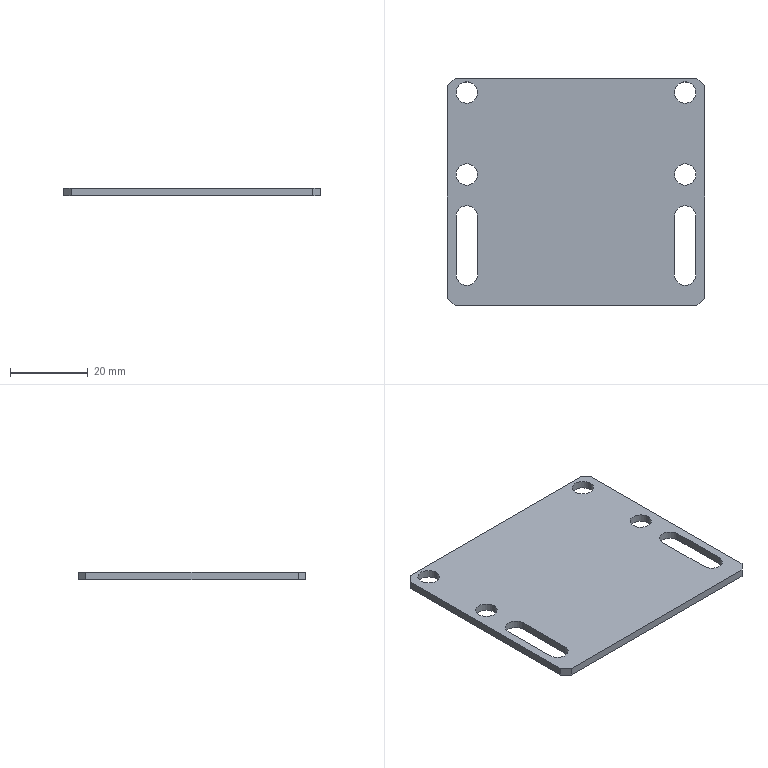Part | STEP file | PN_0001-01-12 Sensor board | 1 solid | 26 faces | box 66 x 58.5 x 2 mm | volume 7091 mm3 | plane 14 | cylinder 12 | commonest cylinder face diameters 5.5 x12
STEP:
#1=CARTESIAN_POINT('',(30.75,4.5,0.));
#2=VERTEX_POINT('',#1);
#3=CARTESIAN_POINT('',(25.25,4.5,0.));
#4=VERTEX_POINT('',#3);
#5=CARTESIAN_POINT('',(28.,4.5,0.));
#6=DIRECTION('',(0.,0.,-1.));
#7=DIRECTION('',(1.,0.,0.));
#8=AXIS2_PLACEMENT_3D('',#5,#6,#7);
#9=CIRCLE('',#8,2.75);
#10=EDGE_CURVE('',#2,#4,#9,.T.);
#11=ORIENTED_EDGE('',*,*,#10,.T.);
#12=CARTESIAN_POINT('',(25.25,4.5,2.));
#13=VERTEX_POINT('',#12);
#14=CARTESIAN_POINT('',(25.25,4.5,-0.001));
#15=DIRECTION('',(0.,0.,1.));
#16=VECTOR('',#15,1000.);
#17=LINE('',#14,#16);
#18=EDGE_CURVE('',#4,#13,#17,.T.);
#19=ORIENTED_EDGE('',*,*,#18,.T.);
#20=CARTESIAN_POINT('',(30.75,4.5,2.));
#21=VERTEX_POINT('',#20);
#22=CARTESIAN_POINT('',(28.,4.5,2.));
#23=DIRECTION('',(0.,0.,1.));
#24=DIRECTION('',(1.,0.,0.));
#25=AXIS2_PLACEMENT_3D('',#22,#23,#24);
#26=CIRCLE('',#25,2.75);
#27=EDGE_CURVE('',#13,#21,#26,.T.);
#28=ORIENTED_EDGE('',*,*,#27,.T.);
#29=CARTESIAN_POINT('',(30.75,4.5,-0.001));
#30=DIRECTION('',(0.,0.,1.));
#31=VECTOR('',#30,1000.);
#32=LINE('',#29,#31);
#33=EDGE_CURVE('',#2,#21,#32,.T.);
#34=ORIENTED_EDGE('',*,*,#33,.F.);
#35=EDGE_LOOP('',(#11,#19,#28,#34));
#36=FACE_OUTER_BOUND('',#35,.T.);
#37=CARTESIAN_POINT('',(28.,4.5,-0.001));
#38=DIRECTION('',(0.,0.,1.));
#39=DIRECTION('',(1.,0.,0.));
#40=AXIS2_PLACEMENT_3D('',#37,#38,#39);
#41=CYLINDRICAL_SURFACE('',#40,2.75);
#42=ADVANCED_FACE('',(#36),#41,.F.);
#43=CARTESIAN_POINT('',(-25.25,4.5,0.));
#44=VERTEX_POINT('',#43);
#45=CARTESIAN_POINT('',(-30.75,4.5,0.));
#46=VERTEX_POINT('',#45);
#47=CARTESIAN_POINT('',(-28.,4.5,0.));
#48=DIRECTION('',(0.,0.,-1.));
#49=DIRECTION('',(1.,0.,0.));
#50=AXIS2_PLACEMENT_3D('',#47,#48,#49);
#51=CIRCLE('',#50,2.75);
#52=EDGE_CURVE('',#44,#46,#51,.T.);
#53=ORIENTED_EDGE('',*,*,#52,.T.);
#54=CARTESIAN_POINT('',(-30.75,4.5,2.));
#55=VERTEX_POINT('',#54);
#56=CARTESIAN_POINT('',(-30.75,4.5,-0.001));
#57=DIRECTION('',(0.,0.,1.));
#58=VECTOR('',#57,1000.);
#59=LINE('',#56,#58);
#60=EDGE_CURVE('',#46,#55,#59,.T.);
#61=ORIENTED_EDGE('',*,*,#60,.T.);
#62=CARTESIAN_POINT('',(-25.25,4.5,2.));
#63=VERTEX_POINT('',#62);
#64=CARTESIAN_POINT('',(-28.,4.5,2.));
#65=DIRECTION('',(0.,0.,1.));
#66=DIRECTION('',(1.,0.,0.));
#67=AXIS2_PLACEMENT_3D('',#64,#65,#66);
#68=CIRCLE('',#67,2.75);
#69=EDGE_CURVE('',#55,#63,#68,.T.);
#70=ORIENTED_EDGE('',*,*,#69,.T.);
#71=CARTESIAN_POINT('',(-25.25,4.5,-0.001));
#72=DIRECTION('',(0.,0.,1.));
#73=VECTOR('',#72,1000.);
#74=LINE('',#71,#73);
#75=EDGE_CURVE('',#44,#63,#74,.T.);
#76=ORIENTED_EDGE('',*,*,#75,.F.);
#77=EDGE_LOOP('',(#53,#61,#70,#76));
#78=FACE_OUTER_BOUND('',#77,.T.);
#79=CARTESIAN_POINT('',(-28.,4.5,-0.001));
#80=DIRECTION('',(0.,0.,1.));
#81=DIRECTION('',(1.,0.,0.));
#82=AXIS2_PLACEMENT_3D('',#79,#80,#81);
#83=CYLINDRICAL_SURFACE('',#82,2.75);
#84=ADVANCED_FACE('',(#78),#83,.F.);
#85=CARTESIAN_POINT('',(30.75,25.5,0.));
#86=VERTEX_POINT('',#85);
#87=CARTESIAN_POINT('',(25.25,25.5,0.));
#88=VERTEX_POINT('',#87);
#89=CARTESIAN_POINT('',(28.,25.5,0.));
#90=DIRECTION('',(0.,0.,-1.));
#91=DIRECTION('',(1.,0.,0.));
#92=AXIS2_PLACEMENT_3D('',#89,#90,#91);
#93=CIRCLE('',#92,2.75);
#94=EDGE_CURVE('',#86,#88,#93,.T.);
#95=ORIENTED_EDGE('',*,*,#94,.T.);
#96=CARTESIAN_POINT('',(25.25,25.5,2.));
#97=VERTEX_POINT('',#96);
#98=CARTESIAN_POINT('',(25.25,25.5,-0.001));
#99=DIRECTION('',(0.,0.,1.));
#100=VECTOR('',#99,1000.);
#101=LINE('',#98,#100);
#102=EDGE_CURVE('',#88,#97,#101,.T.);
#103=ORIENTED_EDGE('',*,*,#102,.T.);
#104=CARTESIAN_POINT('',(30.75,25.5,2.));
#105=VERTEX_POINT('',#104);
#106=CARTESIAN_POINT('',(28.,25.5,2.));
#107=DIRECTION('',(0.,0.,1.));
#108=DIRECTION('',(1.,0.,0.));
#109=AXIS2_PLACEMENT_3D('',#106,#107,#108);
#110=CIRCLE('',#109,2.75);
#111=EDGE_CURVE('',#97,#105,#110,.T.);
#112=ORIENTED_EDGE('',*,*,#111,.T.);
#113=CARTESIAN_POINT('',(30.75,25.5,-0.001));
#114=DIRECTION('',(0.,0.,1.));
#115=VECTOR('',#114,1000.);
#116=LINE('',#113,#115);
#117=EDGE_CURVE('',#86,#105,#116,.T.);
#118=ORIENTED_EDGE('',*,*,#117,.F.);
#119=EDGE_LOOP('',(#95,#103,#112,#118));
#120=FACE_OUTER_BOUND('',#119,.T.);
#121=CARTESIAN_POINT('',(28.,25.5,-0.001));
#122=DIRECTION('',(0.,0.,1.));
#123=DIRECTION('',(1.,0.,0.));
#124=AXIS2_PLACEMENT_3D('',#121,#122,#123);
#125=CYLINDRICAL_SURFACE('',#124,2.75);
#126=ADVANCED_FACE('',(#120),#125,.F.);
#127=CARTESIAN_POINT('',(-25.25,25.5,0.));
#128=VERTEX_POINT('',#127);
#129=CARTESIAN_POINT('',(-30.75,25.5,0.));
#130=VERTEX_POINT('',#129);
#131=CARTESIAN_POINT('',(-28.,25.5,0.));
#132=DIRECTION('',(0.,0.,-1.));
#133=DIRECTION('',(1.,0.,0.));
#134=AXIS2_PLACEMENT_3D('',#131,#132,#133);
#135=CIRCLE('',#134,2.75);
#136=EDGE_CURVE('',#128,#130,#135,.T.);
#137=ORIENTED_EDGE('',*,*,#136,.T.);
#138=CARTESIAN_POINT('',(-30.75,25.5,2.));
#139=VERTEX_POINT('',#138);
#140=CARTESIAN_POINT('',(-30.75,25.5,-0.001));
#141=DIRECTION('',(0.,0.,1.));
#142=VECTOR('',#141,1000.);
#143=LINE('',#140,#142);
#144=EDGE_CURVE('',#130,#139,#143,.T.);
#145=ORIENTED_EDGE('',*,*,#144,.T.);
#146=CARTESIAN_POINT('',(-25.25,25.5,2.));
#147=VERTEX_POINT('',#146);
#148=CARTESIAN_POINT('',(-28.,25.5,2.));
#149=DIRECTION('',(0.,0.,1.));
#150=DIRECTION('',(1.,0.,0.));
#151=AXIS2_PLACEMENT_3D('',#148,#149,#150);
#152=CIRCLE('',#151,2.75);
#153=EDGE_CURVE('',#139,#147,#152,.T.);
#154=ORIENTED_EDGE('',*,*,#153,.T.);
#155=CARTESIAN_POINT('',(-25.25,25.5,-0.001));
#156=DIRECTION('',(0.,0.,1.));
#157=VECTOR('',#156,1000.);
#158=LINE('',#155,#157);
#159=EDGE_CURVE('',#128,#147,#158,.T.);
#160=ORIENTED_EDGE('',*,*,#159,.F.);
#161=EDGE_LOOP('',(#137,#145,#154,#160));
#162=FACE_OUTER_BOUND('',#161,.T.);
#163=CARTESIAN_POINT('',(-28.,25.5,-0.001));
#164=DIRECTION('',(0.,0.,1.));
#165=DIRECTION('',(1.,0.,0.));
#166=AXIS2_PLACEMENT_3D('',#163,#164,#165);
#167=CYLINDRICAL_SURFACE('',#166,2.75);
#168=ADVANCED_FACE('',(#162),#167,.F.);
#169=CARTESIAN_POINT('',(25.25,-21.25,0.));
#170=VERTEX_POINT('',#169);
#171=CARTESIAN_POINT('',(25.25,-21.25,2.));
#172=VERTEX_POINT('',#171);
#173=CARTESIAN_POINT('',(25.25,-21.25,-0.001));
#174=DIRECTION('',(0.,0.,1.));
#175=VECTOR('',#174,1000.);
#176=LINE('',#173,#175);
#177=EDGE_CURVE('',#170,#172,#176,.T.);
#178=ORIENTED_EDGE('',*,*,#177,.T.);
#179=CARTESIAN_POINT('',(30.75,-21.25,2.));
#180=VERTEX_POINT('',#179);
#181=CARTESIAN_POINT('',(28.,-21.25,2.));
#182=DIRECTION('',(0.,0.,1.));
#183=DIRECTION('',(1.,0.,0.));
#184=AXIS2_PLACEMENT_3D('',#181,#182,#183);
#185=CIRCLE('',#184,2.75);
#186=EDGE_CURVE('',#172,#180,#185,.T.);
#187=ORIENTED_EDGE('',*,*,#186,.T.);
#188=CARTESIAN_POINT('',(30.75,-21.25,0.));
#189=VERTEX_POINT('',#188);
#190=CARTESIAN_POINT('',(30.75,-21.25,-0.001));
#191=DIRECTION('',(0.,0.,1.));
#192=VECTOR('',#191,1000.);
#193=LINE('',#190,#192);
#194=EDGE_CURVE('',#189,#180,#193,.T.);
#195=ORIENTED_EDGE('',*,*,#194,.F.);
#196=CARTESIAN_POINT('',(28.,-21.25,0.));
#197=DIRECTION('',(0.,0.,-1.));
#198=DIRECTION('',(1.,0.,0.));
#199=AXIS2_PLACEMENT_3D('',#196,#197,#198);
#200=CIRCLE('',#199,2.75);
#201=EDGE_CURVE('',#189,#170,#200,.T.);
#202=ORIENTED_EDGE('',*,*,#201,.T.);
#203=EDGE_LOOP('',(#178,#187,#195,#202));
#204=FACE_OUTER_BOUND('',#203,.T.);
#205=CARTESIAN_POINT('',(28.,-21.25,-0.001));
#206=DIRECTION('',(0.,0.,1.));
#207=DIRECTION('',(1.,0.,0.));
#208=AXIS2_PLACEMENT_3D('',#205,#206,#207);
#209=CYLINDRICAL_SURFACE('',#208,2.75);
#210=ADVANCED_FACE('',(#204),#209,.F.);
#211=CARTESIAN_POINT('',(-30.75,-21.25,0.));
#212=VERTEX_POINT('',#211);
#213=CARTESIAN_POINT('',(-30.75,-21.25,2.));
#214=VERTEX_POINT('',#213);
#215=CARTESIAN_POINT('',(-30.75,-21.25,-0.001));
#216=DIRECTION('',(0.,0.,1.));
#217=VECTOR('',#216,1000.);
#218=LINE('',#215,#217);
#219=EDGE_CURVE('',#212,#214,#218,.T.);
#220=ORIENTED_EDGE('',*,*,#219,.T.);
#221=CARTESIAN_POINT('',(-25.25,-21.25,2.));
#222=VERTEX_POINT('',#221);
#223=CARTESIAN_POINT('',(-28.,-21.25,2.));
#224=DIRECTION('',(0.,0.,1.));
#225=DIRECTION('',(1.,0.,0.));
#226=AXIS2_PLACEMENT_3D('',#223,#224,#225);
#227=CIRCLE('',#226,2.75);
#228=EDGE_CURVE('',#214,#222,#227,.T.);
#229=ORIENTED_EDGE('',*,*,#228,.T.);
#230=CARTESIAN_POINT('',(-25.25,-21.25,0.));
#231=VERTEX_POINT('',#230);
#232=CARTESIAN_POINT('',(-25.25,-21.25,-0.001));
#233=DIRECTION('',(0.,0.,1.));
#234=VECTOR('',#233,1000.);
#235=LINE('',#232,#234);
#236=EDGE_CURVE('',#231,#222,#235,.T.);
#237=ORIENTED_EDGE('',*,*,#236,.F.);
#238=CARTESIAN_POINT('',(-28.,-21.25,0.));
#239=DIRECTION('',(0.,0.,-1.));
#240=DIRECTION('',(1.,0.,0.));
#241=AXIS2_PLACEMENT_3D('',#238,#239,#240);
#242=CIRCLE('',#241,2.75);
#243=EDGE_CURVE('',#231,#212,#242,.T.);
#244=ORIENTED_EDGE('',*,*,#243,.T.);
#245=EDGE_LOOP('',(#220,#229,#237,#244));
#246=FACE_OUTER_BOUND('',#245,.T.);
#247=CARTESIAN_POINT('',(-28.,-21.25,-0.001));
#248=DIRECTION('',(0.,0.,1.));
#249=DIRECTION('',(1.,0.,0.));
#250=AXIS2_PLACEMENT_3D('',#247,#248,#249);
#251=CYLINDRICAL_SURFACE('',#250,2.75);
#252=ADVANCED_FACE('',(#246),#251,.F.);
#253=CARTESIAN_POINT('',(-33.,27.25,0.));
#254=VERTEX_POINT('',#253);
#255=CARTESIAN_POINT('',(-33.,-27.25,0.));
#256=VERTEX_POINT('',#255);
#257=CARTESIAN_POINT('',(-33.,-29.25,0.));
#258=DIRECTION('',(0.,-1.,0.));
#259=VECTOR('',#258,1000.);
#260=LINE('',#257,#259);
#261=EDGE_CURVE('',#254,#256,#260,.T.);
#262=ORIENTED_EDGE('',*,*,#261,.T.);
#263=CARTESIAN_POINT('',(-33.,-27.25,2.));
#264=VERTEX_POINT('',#263);
#265=CARTESIAN_POINT('',(-33.,-27.25,2.));
#266=DIRECTION('',(0.,0.,1.));
#267=VECTOR('',#266,1000.);
#268=LINE('',#265,#267);
#269=EDGE_CURVE('',#256,#264,#268,.T.);
#270=ORIENTED_EDGE('',*,*,#269,.T.);
#271=CARTESIAN_POINT('',(-33.,27.25,2.));
#272=VERTEX_POINT('',#271);
#273=CARTESIAN_POINT('',(-33.,-29.25,2.));
#274=DIRECTION('',(0.,-1.,0.));
#275=VECTOR('',#274,1000.);
#276=LINE('',#273,#275);
#277=EDGE_CURVE('',#272,#264,#276,.T.);
#278=ORIENTED_EDGE('',*,*,#277,.F.);
#279=CARTESIAN_POINT('',(-33.,27.25,2.));
#280=DIRECTION('',(0.,0.,-1.));
#281=VECTOR('',#280,1000.);
#282=LINE('',#279,#281);
#283=EDGE_CURVE('',#272,#254,#282,.T.);
#284=ORIENTED_EDGE('',*,*,#283,.T.);
#285=EDGE_LOOP('',(#262,#270,#278,#284));
#286=FACE_OUTER_BOUND('',#285,.T.);
#287=CARTESIAN_POINT('',(-33.,-29.25,2.));
#288=DIRECTION('',(1.,0.,0.));
#289=DIRECTION('',(0.,0.,-1.));
#290=AXIS2_PLACEMENT_3D('',#287,#288,#289);
#291=PLANE('',#290);
#292=ADVANCED_FACE('',(#286),#291,.F.);
#293=CARTESIAN_POINT('',(-31.,-29.25,2.));
#294=VERTEX_POINT('',#293);
#295=CARTESIAN_POINT('',(31.,-29.25,2.));
#296=VERTEX_POINT('',#295);
#297=CARTESIAN_POINT('',(33.,-29.25,2.));
#298=DIRECTION('',(1.,0.,0.));
#299=VECTOR('',#298,1000.);
#300=LINE('',#297,#299);
#301=EDGE_CURVE('',#294,#296,#300,.T.);
#302=ORIENTED_EDGE('',*,*,#301,.F.);
#303=CARTESIAN_POINT('',(-31.,-29.25,0.));
#304=VERTEX_POINT('',#303);
#305=CARTESIAN_POINT('',(-31.,-29.25,2.));
#306=DIRECTION('',(0.,0.,-1.));
#307=VECTOR('',#306,1000.);
#308=LINE('',#305,#307);
#309=EDGE_CURVE('',#294,#304,#308,.T.);
#310=ORIENTED_EDGE('',*,*,#309,.T.);
#311=CARTESIAN_POINT('',(31.,-29.25,0.));
#312=VERTEX_POINT('',#311);
#313=CARTESIAN_POINT('',(33.,-29.25,0.));
#314=DIRECTION('',(1.,0.,0.));
#315=VECTOR('',#314,1000.);
#316=LINE('',#313,#315);
#317=EDGE_CURVE('',#304,#312,#316,.T.);
#318=ORIENTED_EDGE('',*,*,#317,.T.);
#319=CARTESIAN_POINT('',(31.,-29.25,2.));
#320=DIRECTION('',(0.,0.,1.));
#321=VECTOR('',#320,1000.);
#322=LINE('',#319,#321);
#323=EDGE_CURVE('',#312,#296,#322,.T.);
#324=ORIENTED_EDGE('',*,*,#323,.T.);
#325=EDGE_LOOP('',(#302,#310,#318,#324));
#326=FACE_OUTER_BOUND('',#325,.T.);
#327=CARTESIAN_POINT('',(33.,-29.25,2.));
#328=DIRECTION('',(0.,1.,0.));
#329=DIRECTION('',(-1.,0.,0.));
#330=AXIS2_PLACEMENT_3D('',#327,#328,#329);
#331=PLANE('',#330);
#332=ADVANCED_FACE('',(#326),#331,.F.);
#333=CARTESIAN_POINT('',(33.,-27.25,2.));
#334=VERTEX_POINT('',#333);
#335=CARTESIAN_POINT('',(33.,27.25,2.));
#336=VERTEX_POINT('',#335);
#337=CARTESIAN_POINT('',(33.,-29.25,2.));
#338=DIRECTION('',(0.,1.,0.));
#339=VECTOR('',#338,1000.);
#340=LINE('',#337,#339);
#341=EDGE_CURVE('',#334,#336,#340,.T.);
#342=ORIENTED_EDGE('',*,*,#341,.F.);
#343=CARTESIAN_POINT('',(33.,-27.25,0.));
#344=VERTEX_POINT('',#343);
#345=CARTESIAN_POINT('',(33.,-27.25,2.));
#346=DIRECTION('',(0.,0.,-1.));
#347=VECTOR('',#346,1000.);
#348=LINE('',#345,#347);
#349=EDGE_CURVE('',#334,#344,#348,.T.);
#350=ORIENTED_EDGE('',*,*,#349,.T.);
#351=CARTESIAN_POINT('',(33.,27.25,0.));
#352=VERTEX_POINT('',#351);
#353=CARTESIAN_POINT('',(33.,-29.25,0.));
#354=DIRECTION('',(0.,1.,0.));
#355=VECTOR('',#354,1000.);
#356=LINE('',#353,#355);
#357=EDGE_CURVE('',#344,#352,#356,.T.);
#358=ORIENTED_EDGE('',*,*,#357,.T.);
#359=CARTESIAN_POINT('',(33.,27.25,2.));
#360=DIRECTION('',(0.,0.,1.));
#361=VECTOR('',#360,1000.);
#362=LINE('',#359,#361);
#363=EDGE_CURVE('',#352,#336,#362,.T.);
#364=ORIENTED_EDGE('',*,*,#363,.T.);
#365=EDGE_LOOP('',(#342,#350,#358,#364));
#366=FACE_OUTER_BOUND('',#365,.T.);
#367=CARTESIAN_POINT('',(33.,-29.25,2.));
#368=DIRECTION('',(-1.,0.,0.));
#369=DIRECTION('',(0.,0.,1.));
#370=AXIS2_PLACEMENT_3D('',#367,#368,#369);
#371=PLANE('',#370);
#372=ADVANCED_FACE('',(#366),#371,.F.);
#373=CARTESIAN_POINT('',(31.,29.25,0.));
#374=VERTEX_POINT('',#373);
#375=CARTESIAN_POINT('',(-31.,29.25,0.));
#376=VERTEX_POINT('',#375);
#377=CARTESIAN_POINT('',(33.,29.25,0.));
#378=DIRECTION('',(-1.,0.,0.));
#379=VECTOR('',#378,1000.);
#380=LINE('',#377,#379);
#381=EDGE_CURVE('',#374,#376,#380,.T.);
#382=ORIENTED_EDGE('',*,*,#381,.T.);
#383=CARTESIAN_POINT('',(-31.,29.25,2.));
#384=VERTEX_POINT('',#383);
#385=CARTESIAN_POINT('',(-31.,29.25,2.));
#386=DIRECTION('',(0.,0.,1.));
#387=VECTOR('',#386,1000.);
#388=LINE('',#385,#387);
#389=EDGE_CURVE('',#376,#384,#388,.T.);
#390=ORIENTED_EDGE('',*,*,#389,.T.);
#391=CARTESIAN_POINT('',(31.,29.25,2.));
#392=VERTEX_POINT('',#391);
#393=CARTESIAN_POINT('',(33.,29.25,2.));
#394=DIRECTION('',(-1.,0.,0.));
#395=VECTOR('',#394,1000.);
#396=LINE('',#393,#395);
#397=EDGE_CURVE('',#392,#384,#396,.T.);
#398=ORIENTED_EDGE('',*,*,#397,.F.);
#399=CARTESIAN_POINT('',(31.,29.25,2.));
#400=DIRECTION('',(0.,0.,-1.));
#401=VECTOR('',#400,1000.);
#402=LINE('',#399,#401);
#403=EDGE_CURVE('',#392,#374,#402,.T.);
#404=ORIENTED_EDGE('',*,*,#403,.T.);
#405=EDGE_LOOP('',(#382,#390,#398,#404));
#406=FACE_OUTER_BOUND('',#405,.T.);
#407=CARTESIAN_POINT('',(33.,29.25,2.));
#408=DIRECTION('',(0.,-1.,0.));
#409=DIRECTION('',(1.,0.,0.));
#410=AXIS2_PLACEMENT_3D('',#407,#408,#409);
#411=PLANE('',#410);
#412=ADVANCED_FACE('',(#406),#411,.F.);
#413=CARTESIAN_POINT('',(-30.75,-6.25,2.));
#414=VERTEX_POINT('',#413);
#415=CARTESIAN_POINT('',(-30.75,-21.25,2.));
#416=DIRECTION('',(0.,-1.,0.));
#417=VECTOR('',#416,1000.);
#418=LINE('',#415,#417);
#419=EDGE_CURVE('',#414,#214,#418,.T.);
#420=ORIENTED_EDGE('',*,*,#419,.F.);
#421=CARTESIAN_POINT('',(-25.25,-6.25,2.));
#422=VERTEX_POINT('',#421);
#423=CARTESIAN_POINT('',(-28.,-6.25,2.));
#424=DIRECTION('',(0.,0.,1.));
#425=DIRECTION('',(1.,0.,0.));
#426=AXIS2_PLACEMENT_3D('',#423,#424,#425);
#427=CIRCLE('',#426,2.75);
#428=EDGE_CURVE('',#422,#414,#427,.T.);
#429=ORIENTED_EDGE('',*,*,#428,.F.);
#430=CARTESIAN_POINT('',(-25.25,-21.25,2.));
#431=DIRECTION('',(0.,1.,0.));
#432=VECTOR('',#431,1000.);
#433=LINE('',#430,#432);
#434=EDGE_CURVE('',#222,#422,#433,.T.);
#435=ORIENTED_EDGE('',*,*,#434,.F.);
#436=ORIENTED_EDGE('',*,*,#228,.F.);
#437=EDGE_LOOP('',(#420,#429,#435,#436));
#438=FACE_BOUND('',#437,.T.);
#439=CARTESIAN_POINT('',(25.25,-6.25,2.));
#440=VERTEX_POINT('',#439);
#441=CARTESIAN_POINT('',(25.25,-21.25,2.));
#442=DIRECTION('',(0.,-1.,0.));
#443=VECTOR('',#442,1000.);
#444=LINE('',#441,#443);
#445=EDGE_CURVE('',#440,#172,#444,.T.);
#446=ORIENTED_EDGE('',*,*,#445,.F.);
#447=CARTESIAN_POINT('',(30.75,-6.25,2.));
#448=VERTEX_POINT('',#447);
#449=CARTESIAN_POINT('',(28.,-6.25,2.));
#450=DIRECTION('',(0.,0.,1.));
#451=DIRECTION('',(1.,0.,0.));
#452=AXIS2_PLACEMENT_3D('',#449,#450,#451);
#453=CIRCLE('',#452,2.75);
#454=EDGE_CURVE('',#448,#440,#453,.T.);
#455=ORIENTED_EDGE('',*,*,#454,.F.);
#456=CARTESIAN_POINT('',(30.75,-21.25,2.));
#457=DIRECTION('',(0.,1.,0.));
#458=VECTOR('',#457,1000.);
#459=LINE('',#456,#458);
#460=EDGE_CURVE('',#180,#448,#459,.T.);
#461=ORIENTED_EDGE('',*,*,#460,.F.);
#462=ORIENTED_EDGE('',*,*,#186,.F.);
#463=EDGE_LOOP('',(#446,#455,#461,#462));
#464=FACE_BOUND('',#463,.T.);
#465=CARTESIAN_POINT('',(28.,4.5,2.));
#466=DIRECTION('',(0.,0.,1.));
#467=DIRECTION('',(1.,0.,0.));
#468=AXIS2_PLACEMENT_3D('',#465,#466,#467);
#469=CIRCLE('',#468,2.75);
#470=EDGE_CURVE('',#21,#13,#469,.T.);
#471=ORIENTED_EDGE('',*,*,#470,.F.);
#472=ORIENTED_EDGE('',*,*,#27,.F.);
#473=EDGE_LOOP('',(#471,#472));
#474=FACE_BOUND('',#473,.T.);
#475=CARTESIAN_POINT('',(-28.,4.5,2.));
#476=DIRECTION('',(0.,0.,1.));
#477=DIRECTION('',(1.,0.,0.));
#478=AXIS2_PLACEMENT_3D('',#475,#476,#477);
#479=CIRCLE('',#478,2.75);
#480=EDGE_CURVE('',#63,#55,#479,.T.);
#481=ORIENTED_EDGE('',*,*,#480,.F.);
#482=ORIENTED_EDGE('',*,*,#69,.F.);
#483=EDGE_LOOP('',(#481,#482));
#484=FACE_BOUND('',#483,.T.);
#485=CARTESIAN_POINT('',(28.,25.5,2.));
#486=DIRECTION('',(0.,0.,1.));
#487=DIRECTION('',(1.,0.,0.));
#488=AXIS2_PLACEMENT_3D('',#485,#486,#487);
#489=CIRCLE('',#488,2.75);
#490=EDGE_CURVE('',#105,#97,#489,.T.);
#491=ORIENTED_EDGE('',*,*,#490,.F.);
#492=ORIENTED_EDGE('',*,*,#111,.F.);
#493=EDGE_LOOP('',(#491,#492));
#494=FACE_BOUND('',#493,.T.);
#495=CARTESIAN_POINT('',(-28.,25.5,2.));
#496=DIRECTION('',(0.,0.,1.));
#497=DIRECTION('',(1.,0.,0.));
#498=AXIS2_PLACEMENT_3D('',#495,#496,#497);
#499=CIRCLE('',#498,2.75);
#500=EDGE_CURVE('',#147,#139,#499,.T.);
#501=ORIENTED_EDGE('',*,*,#500,.F.);
#502=ORIENTED_EDGE('',*,*,#153,.F.);
#503=EDGE_LOOP('',(#501,#502));
#504=FACE_BOUND('',#503,.T.);
#505=ORIENTED_EDGE('',*,*,#277,.T.);
#506=CARTESIAN_POINT('',(-30.125,-30.125,2.));
#507=DIRECTION('',(0.7071,-0.7071,0.));
#508=VECTOR('',#507,1000.);
#509=LINE('',#506,#508);
#510=EDGE_CURVE('',#264,#294,#509,.T.);
#511=ORIENTED_EDGE('',*,*,#510,.T.);
#512=ORIENTED_EDGE('',*,*,#301,.T.);
#513=CARTESIAN_POINT('',(30.125,-30.125,2.));
#514=DIRECTION('',(0.7071,0.7071,0.));
#515=VECTOR('',#514,1000.);
#516=LINE('',#513,#515);
#517=EDGE_CURVE('',#296,#334,#516,.T.);
#518=ORIENTED_EDGE('',*,*,#517,.T.);
#519=ORIENTED_EDGE('',*,*,#341,.T.);
#520=CARTESIAN_POINT('',(30.125,30.125,2.));
#521=DIRECTION('',(-0.7071,0.7071,0.));
#522=VECTOR('',#521,1000.);
#523=LINE('',#520,#522);
#524=EDGE_CURVE('',#336,#392,#523,.T.);
#525=ORIENTED_EDGE('',*,*,#524,.T.);
#526=ORIENTED_EDGE('',*,*,#397,.T.);
#527=CARTESIAN_POINT('',(-30.125,30.125,2.));
#528=DIRECTION('',(-0.7071,-0.7071,0.));
#529=VECTOR('',#528,1000.);
#530=LINE('',#527,#529);
#531=EDGE_CURVE('',#384,#272,#530,.T.);
#532=ORIENTED_EDGE('',*,*,#531,.T.);
#533=EDGE_LOOP('',(#505,#511,#512,#518,#519,#525,#526,#532));
#534=FACE_OUTER_BOUND('',#533,.T.);
#535=CARTESIAN_POINT('',(0.,0.,2.));
#536=DIRECTION('',(0.,0.,1.));
#537=DIRECTION('',(1.,0.,0.));
#538=AXIS2_PLACEMENT_3D('',#535,#536,#537);
#539=PLANE('',#538);
#540=ADVANCED_FACE('',(#438,#464,#474,#484,#494,#504,#534),#539,.T.);
#541=CARTESIAN_POINT('',(-30.75,-6.25,0.));
#542=VERTEX_POINT('',#541);
#543=CARTESIAN_POINT('',(-25.25,-6.25,0.));
#544=VERTEX_POINT('',#543);
#545=CARTESIAN_POINT('',(-28.,-6.25,0.));
#546=DIRECTION('',(0.,0.,-1.));
#547=DIRECTION('',(1.,0.,0.));
#548=AXIS2_PLACEMENT_3D('',#545,#546,#547);
#549=CIRCLE('',#548,2.75);
#550=EDGE_CURVE('',#542,#544,#549,.T.);
#551=ORIENTED_EDGE('',*,*,#550,.F.);
#552=CARTESIAN_POINT('',(-30.75,-21.25,0.));
#553=DIRECTION('',(0.,1.,0.));
#554=VECTOR('',#553,1000.);
#555=LINE('',#552,#554);
#556=EDGE_CURVE('',#212,#542,#555,.T.);
#557=ORIENTED_EDGE('',*,*,#556,.F.);
#558=ORIENTED_EDGE('',*,*,#243,.F.);
#559=CARTESIAN_POINT('',(-25.25,-21.25,0.));
#560=DIRECTION('',(0.,-1.,0.));
#561=VECTOR('',#560,1000.);
#562=LINE('',#559,#561);
#563=EDGE_CURVE('',#544,#231,#562,.T.);
#564=ORIENTED_EDGE('',*,*,#563,.F.);
#565=EDGE_LOOP('',(#551,#557,#558,#564));
#566=FACE_BOUND('',#565,.T.);
#567=ORIENTED_EDGE('',*,*,#10,.F.);
#568=CARTESIAN_POINT('',(28.,4.5,0.));
#569=DIRECTION('',(0.,0.,-1.));
#570=DIRECTION('',(1.,0.,0.));
#571=AXIS2_PLACEMENT_3D('',#568,#569,#570);
#572=CIRCLE('',#571,2.75);
#573=EDGE_CURVE('',#4,#2,#572,.T.);
#574=ORIENTED_EDGE('',*,*,#573,.F.);
#575=EDGE_LOOP('',(#567,#574));
#576=FACE_BOUND('',#575,.T.);
#577=ORIENTED_EDGE('',*,*,#52,.F.);
#578=CARTESIAN_POINT('',(-28.,4.5,0.));
#579=DIRECTION('',(0.,0.,-1.));
#580=DIRECTION('',(1.,0.,0.));
#581=AXIS2_PLACEMENT_3D('',#578,#579,#580);
#582=CIRCLE('',#581,2.75);
#583=EDGE_CURVE('',#46,#44,#582,.T.);
#584=ORIENTED_EDGE('',*,*,#583,.F.);
#585=EDGE_LOOP('',(#577,#584));
#586=FACE_BOUND('',#585,.T.);
#587=ORIENTED_EDGE('',*,*,#94,.F.);
#588=CARTESIAN_POINT('',(28.,25.5,0.));
#589=DIRECTION('',(0.,0.,-1.));
#590=DIRECTION('',(1.,0.,0.));
#591=AXIS2_PLACEMENT_3D('',#588,#589,#590);
#592=CIRCLE('',#591,2.75);
#593=EDGE_CURVE('',#88,#86,#592,.T.);
#594=ORIENTED_EDGE('',*,*,#593,.F.);
#595=EDGE_LOOP('',(#587,#594));
#596=FACE_BOUND('',#595,.T.);
#597=CARTESIAN_POINT('',(25.25,-6.25,0.));
#598=VERTEX_POINT('',#597);
#599=CARTESIAN_POINT('',(30.75,-6.25,0.));
#600=VERTEX_POINT('',#599);
#601=CARTESIAN_POINT('',(28.,-6.25,0.));
#602=DIRECTION('',(0.,0.,-1.));
#603=DIRECTION('',(1.,0.,0.));
#604=AXIS2_PLACEMENT_3D('',#601,#602,#603);
#605=CIRCLE('',#604,2.75);
#606=EDGE_CURVE('',#598,#600,#605,.T.);
#607=ORIENTED_EDGE('',*,*,#606,.F.);
#608=CARTESIAN_POINT('',(25.25,-21.25,0.));
#609=DIRECTION('',(0.,1.,0.));
#610=VECTOR('',#609,1000.);
#611=LINE('',#608,#610);
#612=EDGE_CURVE('',#170,#598,#611,.T.);
#613=ORIENTED_EDGE('',*,*,#612,.F.);
#614=ORIENTED_EDGE('',*,*,#201,.F.);
#615=CARTESIAN_POINT('',(30.75,-21.25,0.));
#616=DIRECTION('',(0.,-1.,0.));
#617=VECTOR('',#616,1000.);
#618=LINE('',#615,#617);
#619=EDGE_CURVE('',#600,#189,#618,.T.);
#620=ORIENTED_EDGE('',*,*,#619,.F.);
#621=EDGE_LOOP('',(#607,#613,#614,#620));
#622=FACE_BOUND('',#621,.T.);
#623=ORIENTED_EDGE('',*,*,#136,.F.);
#624=CARTESIAN_POINT('',(-28.,25.5,0.));
#625=DIRECTION('',(0.,0.,-1.));
#626=DIRECTION('',(1.,0.,0.));
#627=AXIS2_PLACEMENT_3D('',#624,#625,#626);
#628=CIRCLE('',#627,2.75);
#629=EDGE_CURVE('',#130,#128,#628,.T.);
#630=ORIENTED_EDGE('',*,*,#629,.F.);
#631=EDGE_LOOP('',(#623,#630));
#632=FACE_BOUND('',#631,.T.);
#633=ORIENTED_EDGE('',*,*,#317,.F.);
#634=CARTESIAN_POINT('',(-31.,-29.25,0.));
#635=DIRECTION('',(-0.7071,0.7071,0.));
#636=VECTOR('',#635,1000.);
#637=LINE('',#634,#636);
#638=EDGE_CURVE('',#304,#256,#637,.T.);
#639=ORIENTED_EDGE('',*,*,#638,.T.);
#640=ORIENTED_EDGE('',*,*,#261,.F.);
#641=CARTESIAN_POINT('',(-33.,27.25,0.));
#642=DIRECTION('',(0.7071,0.7071,0.));
#643=VECTOR('',#642,1000.);
#644=LINE('',#641,#643);
#645=EDGE_CURVE('',#254,#376,#644,.T.);
#646=ORIENTED_EDGE('',*,*,#645,.T.);
#647=ORIENTED_EDGE('',*,*,#381,.F.);
#648=CARTESIAN_POINT('',(31.,29.25,0.));
#649=DIRECTION('',(0.7071,-0.7071,0.));
#650=VECTOR('',#649,1000.);
#651=LINE('',#648,#650);
#652=EDGE_CURVE('',#374,#352,#651,.T.);
#653=ORIENTED_EDGE('',*,*,#652,.T.);
#654=ORIENTED_EDGE('',*,*,#357,.F.);
#655=CARTESIAN_POINT('',(33.,-27.25,0.));
#656=DIRECTION('',(-0.7071,-0.7071,0.));
#657=VECTOR('',#656,1000.);
#658=LINE('',#655,#657);
#659=EDGE_CURVE('',#344,#312,#658,.T.);
#660=ORIENTED_EDGE('',*,*,#659,.T.);
#661=EDGE_LOOP('',(#633,#639,#640,#646,#647,#653,#654,#660));
#662=FACE_OUTER_BOUND('',#661,.T.);
#663=CARTESIAN_POINT('',(0.,0.,0.));
#664=DIRECTION('',(0.,0.,1.));
#665=DIRECTION('',(1.,0.,0.));
#666=AXIS2_PLACEMENT_3D('',#663,#664,#665);
#667=PLANE('',#666);
#668=ADVANCED_FACE('',(#566,#576,#586,#596,#622,#632,#662),#667,.F.);
#669=ORIENTED_EDGE('',*,*,#510,.F.);
#670=ORIENTED_EDGE('',*,*,#269,.F.);
#671=ORIENTED_EDGE('',*,*,#638,.F.);
#672=ORIENTED_EDGE('',*,*,#309,.F.);
#673=EDGE_LOOP('',(#669,#670,#671,#672));
#674=FACE_OUTER_BOUND('',#673,.T.);
#675=CARTESIAN_POINT('',(-31.,-29.25,2.));
#676=DIRECTION('',(0.7071,0.7071,0.));
#677=DIRECTION('',(0.,0.,-1.));
#678=AXIS2_PLACEMENT_3D('',#675,#676,#677);
#679=PLANE('',#678);
#680=ADVANCED_FACE('',(#674),#679,.F.);
#681=ORIENTED_EDGE('',*,*,#517,.F.);
#682=ORIENTED_EDGE('',*,*,#323,.F.);
#683=ORIENTED_EDGE('',*,*,#659,.F.);
#684=ORIENTED_EDGE('',*,*,#349,.F.);
#685=EDGE_LOOP('',(#681,#682,#683,#684));
#686=FACE_OUTER_BOUND('',#685,.T.);
#687=CARTESIAN_POINT('',(33.,-27.25,2.));
#688=DIRECTION('',(-0.7071,0.7071,0.));
#689=DIRECTION('',(0.,0.,-1.));
#690=AXIS2_PLACEMENT_3D('',#687,#688,#689);
#691=PLANE('',#690);
#692=ADVANCED_FACE('',(#686),#691,.F.);
#693=ORIENTED_EDGE('',*,*,#531,.F.);
#694=ORIENTED_EDGE('',*,*,#389,.F.);
#695=ORIENTED_EDGE('',*,*,#645,.F.);
#696=ORIENTED_EDGE('',*,*,#283,.F.);
#697=EDGE_LOOP('',(#693,#694,#695,#696));
#698=FACE_OUTER_BOUND('',#697,.T.);
#699=CARTESIAN_POINT('',(-33.,27.25,2.));
#700=DIRECTION('',(0.7071,-0.7071,0.));
#701=DIRECTION('',(0.,0.,-1.));
#702=AXIS2_PLACEMENT_3D('',#699,#700,#701);
#703=PLANE('',#702);
#704=ADVANCED_FACE('',(#698),#703,.F.);
#705=ORIENTED_EDGE('',*,*,#524,.F.);
#706=ORIENTED_EDGE('',*,*,#363,.F.);
#707=ORIENTED_EDGE('',*,*,#652,.F.);
#708=ORIENTED_EDGE('',*,*,#403,.F.);
#709=EDGE_LOOP('',(#705,#706,#707,#708));
#710=FACE_OUTER_BOUND('',#709,.T.);
#711=CARTESIAN_POINT('',(31.,29.25,2.));
#712=DIRECTION('',(-0.7071,-0.7071,0.));
#713=DIRECTION('',(0.,0.,-1.));
#714=AXIS2_PLACEMENT_3D('',#711,#712,#713);
#715=PLANE('',#714);
#716=ADVANCED_FACE('',(#710),#715,.F.);
#717=ORIENTED_EDGE('',*,*,#144,.F.);
#718=ORIENTED_EDGE('',*,*,#629,.T.);
#719=ORIENTED_EDGE('',*,*,#159,.T.);
#720=ORIENTED_EDGE('',*,*,#500,.T.);
#721=EDGE_LOOP('',(#717,#718,#719,#720));
#722=FACE_OUTER_BOUND('',#721,.T.);
#723=CARTESIAN_POINT('',(-28.,25.5,-0.001));
#724=DIRECTION('',(0.,0.,1.));
#725=DIRECTION('',(1.,0.,0.));
#726=AXIS2_PLACEMENT_3D('',#723,#724,#725);
#727=CYLINDRICAL_SURFACE('',#726,2.75);
#728=ADVANCED_FACE('',(#722),#727,.F.);
#729=ORIENTED_EDGE('',*,*,#102,.F.);
#730=ORIENTED_EDGE('',*,*,#593,.T.);
#731=ORIENTED_EDGE('',*,*,#117,.T.);
#732=ORIENTED_EDGE('',*,*,#490,.T.);
#733=EDGE_LOOP('',(#729,#730,#731,#732));
#734=FACE_OUTER_BOUND('',#733,.T.);
#735=CARTESIAN_POINT('',(28.,25.5,-0.001));
#736=DIRECTION('',(0.,0.,1.));
#737=DIRECTION('',(1.,0.,0.));
#738=AXIS2_PLACEMENT_3D('',#735,#736,#737);
#739=CYLINDRICAL_SURFACE('',#738,2.75);
#740=ADVANCED_FACE('',(#734),#739,.F.);
#741=ORIENTED_EDGE('',*,*,#60,.F.);
#742=ORIENTED_EDGE('',*,*,#583,.T.);
#743=ORIENTED_EDGE('',*,*,#75,.T.);
#744=ORIENTED_EDGE('',*,*,#480,.T.);
#745=EDGE_LOOP('',(#741,#742,#743,#744));
#746=FACE_OUTER_BOUND('',#745,.T.);
#747=CARTESIAN_POINT('',(-28.,4.5,-0.001));
#748=DIRECTION('',(0.,0.,1.));
#749=DIRECTION('',(1.,0.,0.));
#750=AXIS2_PLACEMENT_3D('',#747,#748,#749);
#751=CYLINDRICAL_SURFACE('',#750,2.75);
#752=ADVANCED_FACE('',(#746),#751,.F.);
#753=ORIENTED_EDGE('',*,*,#18,.F.);
#754=ORIENTED_EDGE('',*,*,#573,.T.);
#755=ORIENTED_EDGE('',*,*,#33,.T.);
#756=ORIENTED_EDGE('',*,*,#470,.T.);
#757=EDGE_LOOP('',(#753,#754,#755,#756));
#758=FACE_OUTER_BOUND('',#757,.T.);
#759=CARTESIAN_POINT('',(28.,4.5,-0.001));
#760=DIRECTION('',(0.,0.,1.));
#761=DIRECTION('',(1.,0.,0.));
#762=AXIS2_PLACEMENT_3D('',#759,#760,#761);
#763=CYLINDRICAL_SURFACE('',#762,2.75);
#764=ADVANCED_FACE('',(#758),#763,.F.);
#765=ORIENTED_EDGE('',*,*,#556,.T.);
#766=CARTESIAN_POINT('',(-30.75,-6.25,-0.001));
#767=DIRECTION('',(0.,0.,1.));
#768=VECTOR('',#767,1000.);
#769=LINE('',#766,#768);
#770=EDGE_CURVE('',#542,#414,#769,.T.);
#771=ORIENTED_EDGE('',*,*,#770,.T.);
#772=ORIENTED_EDGE('',*,*,#419,.T.);
#773=ORIENTED_EDGE('',*,*,#219,.F.);
#774=EDGE_LOOP('',(#765,#771,#772,#773));
#775=FACE_OUTER_BOUND('',#774,.T.);
#776=CARTESIAN_POINT('',(-30.75,-21.25,-0.001));
#777=DIRECTION('',(-1.,0.,0.));
#778=DIRECTION('',(0.,0.,1.));
#779=AXIS2_PLACEMENT_3D('',#776,#777,#778);
#780=PLANE('',#779);
#781=ADVANCED_FACE('',(#775),#780,.F.);
#782=ORIENTED_EDGE('',*,*,#550,.T.);
#783=CARTESIAN_POINT('',(-25.25,-6.25,-0.001));
#784=DIRECTION('',(0.,0.,1.));
#785=VECTOR('',#784,1000.);
#786=LINE('',#783,#785);
#787=EDGE_CURVE('',#544,#422,#786,.T.);
#788=ORIENTED_EDGE('',*,*,#787,.T.);
#789=ORIENTED_EDGE('',*,*,#428,.T.);
#790=ORIENTED_EDGE('',*,*,#770,.F.);
#791=EDGE_LOOP('',(#782,#788,#789,#790));
#792=FACE_OUTER_BOUND('',#791,.T.);
#793=CARTESIAN_POINT('',(-28.,-6.25,-0.001));
#794=DIRECTION('',(0.,0.,1.));
#795=DIRECTION('',(1.,0.,0.));
#796=AXIS2_PLACEMENT_3D('',#793,#794,#795);
#797=CYLINDRICAL_SURFACE('',#796,2.75);
#798=ADVANCED_FACE('',(#792),#797,.F.);
#799=ORIENTED_EDGE('',*,*,#563,.T.);
#800=ORIENTED_EDGE('',*,*,#236,.T.);
#801=ORIENTED_EDGE('',*,*,#434,.T.);
#802=ORIENTED_EDGE('',*,*,#787,.F.);
#803=EDGE_LOOP('',(#799,#800,#801,#802));
#804=FACE_OUTER_BOUND('',#803,.T.);
#805=CARTESIAN_POINT('',(-25.25,-21.25,-0.001));
#806=DIRECTION('',(1.,0.,0.));
#807=DIRECTION('',(0.,0.,-1.));
#808=AXIS2_PLACEMENT_3D('',#805,#806,#807);
#809=PLANE('',#808);
#810=ADVANCED_FACE('',(#804),#809,.F.);
#811=ORIENTED_EDGE('',*,*,#612,.T.);
#812=CARTESIAN_POINT('',(25.25,-6.25,-0.001));
#813=DIRECTION('',(0.,0.,1.));
#814=VECTOR('',#813,1000.);
#815=LINE('',#812,#814);
#816=EDGE_CURVE('',#598,#440,#815,.T.);
#817=ORIENTED_EDGE('',*,*,#816,.T.);
#818=ORIENTED_EDGE('',*,*,#445,.T.);
#819=ORIENTED_EDGE('',*,*,#177,.F.);
#820=EDGE_LOOP('',(#811,#817,#818,#819));
#821=FACE_OUTER_BOUND('',#820,.T.);
#822=CARTESIAN_POINT('',(25.25,-21.25,-0.001));
#823=DIRECTION('',(-1.,0.,0.));
#824=DIRECTION('',(0.,0.,1.));
#825=AXIS2_PLACEMENT_3D('',#822,#823,#824);
#826=PLANE('',#825);
#827=ADVANCED_FACE('',(#821),#826,.F.);
#828=ORIENTED_EDGE('',*,*,#606,.T.);
#829=CARTESIAN_POINT('',(30.75,-6.25,-0.001));
#830=DIRECTION('',(0.,0.,1.));
#831=VECTOR('',#830,1000.);
#832=LINE('',#829,#831);
#833=EDGE_CURVE('',#600,#448,#832,.T.);
#834=ORIENTED_EDGE('',*,*,#833,.T.);
#835=ORIENTED_EDGE('',*,*,#454,.T.);
#836=ORIENTED_EDGE('',*,*,#816,.F.);
#837=EDGE_LOOP('',(#828,#834,#835,#836));
#838=FACE_OUTER_BOUND('',#837,.T.);
#839=CARTESIAN_POINT('',(28.,-6.25,-0.001));
#840=DIRECTION('',(0.,0.,1.));
#841=DIRECTION('',(1.,0.,0.));
#842=AXIS2_PLACEMENT_3D('',#839,#840,#841);
#843=CYLINDRICAL_SURFACE('',#842,2.75);
#844=ADVANCED_FACE('',(#838),#843,.F.);
#845=ORIENTED_EDGE('',*,*,#619,.T.);
#846=ORIENTED_EDGE('',*,*,#194,.T.);
#847=ORIENTED_EDGE('',*,*,#460,.T.);
#848=ORIENTED_EDGE('',*,*,#833,.F.);
#849=EDGE_LOOP('',(#845,#846,#847,#848));
#850=FACE_OUTER_BOUND('',#849,.T.);
#851=CARTESIAN_POINT('',(30.75,-21.25,-0.001));
#852=DIRECTION('',(1.,0.,0.));
#853=DIRECTION('',(0.,0.,-1.));
#854=AXIS2_PLACEMENT_3D('',#851,#852,#853);
#855=PLANE('',#854);
#856=ADVANCED_FACE('',(#850),#855,.F.);
#857=CLOSED_SHELL('',(#42,#84,#126,#168,#210,#252,#292,#332,#372,#412,#540,#668,#680,#692,#704,#716,#728,#740,#752,#764,#781,#798,#810,#827,#844,#856));
#858=MANIFOLD_SOLID_BREP('',#857);
#859=CARTESIAN_POINT('',(0.,0.,0.));
#860=DIRECTION('',(0.,0.,1.));
#861=DIRECTION('',(1.,0.,0.));
#862=AXIS2_PLACEMENT_3D('',#859,#860,#861);
#863=(LENGTH_UNIT()NAMED_UNIT(*)SI_UNIT(.MILLI.,.METRE.));
#864=UNCERTAINTY_MEASURE_WITH_UNIT(LENGTH_MEASURE(0.00001),#863,'','');
#865=(NAMED_UNIT(*)PLANE_ANGLE_UNIT()SI_UNIT($,.RADIAN.));
#866=(NAMED_UNIT(*)SI_UNIT($,.STERADIAN.)SOLID_ANGLE_UNIT());
#867=(GEOMETRIC_REPRESENTATION_CONTEXT(3)GLOBAL_UNCERTAINTY_ASSIGNED_CONTEXT((#864))GLOBAL_UNIT_ASSIGNED_CONTEXT((#863,#865,#866))REPRESENTATION_CONTEXT('',''));
#868=ADVANCED_BREP_SHAPE_REPRESENTATION('',(#858,#862),#867);